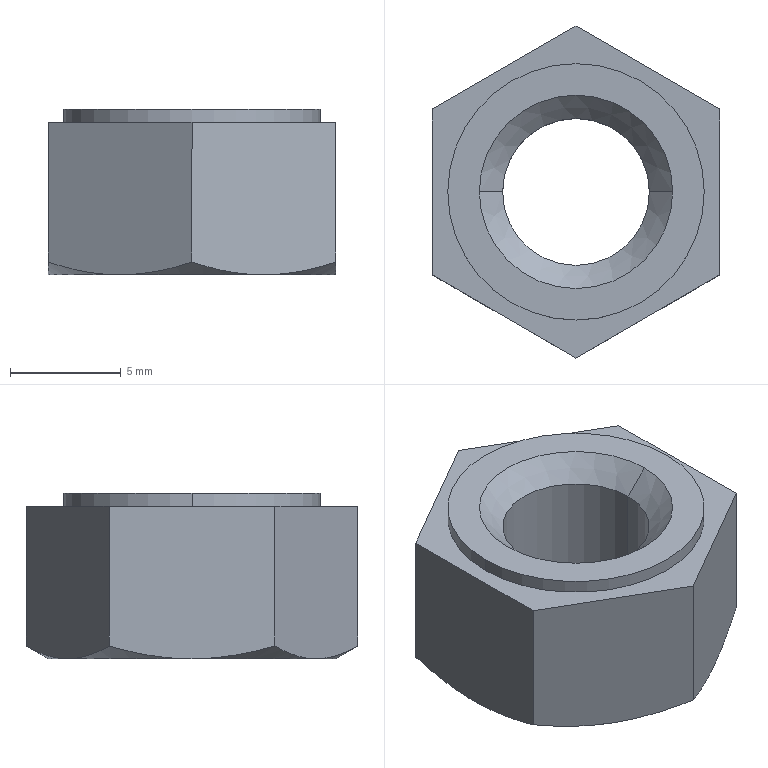Part | SolidWorks | features BaseBody 1 | 1 solid | 23 faces | box 13 x 15.011 x 7.5 mm | volume 785.095 mm3 | cone 10 | plane 9 | cylinder 4 | commonest cylinder face diameters 6.647 x2 11.6 x2
STEP:
#1=CARTESIAN_POINT('',(3.323,0.,1.052));
#2=VERTEX_POINT('',#1);
#3=CARTESIAN_POINT('',(-3.323,0.,1.052));
#4=VERTEX_POINT('',#3);
#5=CARTESIAN_POINT('',(0.,0.,1.052));
#6=DIRECTION('',(0.,0.,-1.));
#7=DIRECTION('',(-1.,0.,0.));
#8=AXIS2_PLACEMENT_3D('',#5,#6,#7);
#9=CIRCLE('',#8,3.323);
#10=EDGE_CURVE('',#2,#4,#9,.T.);
#11=ORIENTED_EDGE('',*,*,#10,.F.);
#12=CARTESIAN_POINT('',(4.375,0.,0.));
#13=VERTEX_POINT('',#12);
#14=CARTESIAN_POINT('',(4.375,0.,0.));
#15=DIRECTION('',(0.7071,0.,-0.7071));
#16=VECTOR('',#15,1000.);
#17=LINE('',#14,#16);
#18=EDGE_CURVE('',#2,#13,#17,.T.);
#19=ORIENTED_EDGE('',*,*,#18,.T.);
#20=CARTESIAN_POINT('',(-4.375,0.,0.));
#21=VERTEX_POINT('',#20);
#22=CARTESIAN_POINT('',(0.,0.,0.));
#23=DIRECTION('',(0.,0.,1.));
#24=DIRECTION('',(-1.,0.,0.));
#25=AXIS2_PLACEMENT_3D('',#22,#23,#24);
#26=CIRCLE('',#25,4.375);
#27=EDGE_CURVE('',#21,#13,#26,.T.);
#28=ORIENTED_EDGE('',*,*,#27,.F.);
#29=CARTESIAN_POINT('',(-4.375,0.,0.));
#30=DIRECTION('',(-0.7071,0.,-0.7071));
#31=VECTOR('',#30,1000.);
#32=LINE('',#29,#31);
#33=EDGE_CURVE('',#4,#21,#32,.T.);
#34=ORIENTED_EDGE('',*,*,#33,.F.);
#35=EDGE_LOOP('',(#11,#19,#28,#34));
#36=FACE_OUTER_BOUND('',#35,.T.);
#37=CARTESIAN_POINT('',(0.,0.,0.));
#38=DIRECTION('',(0.,0.,-1.));
#39=DIRECTION('',(-1.,0.,0.));
#40=AXIS2_PLACEMENT_3D('',#37,#38,#39);
#41=CONICAL_SURFACE('',#40,4.375,0.7854);
#42=ADVANCED_FACE('',(#36),#41,.F.);
#43=CARTESIAN_POINT('',(3.323,0.,6.448));
#44=VERTEX_POINT('',#43);
#45=CARTESIAN_POINT('',(-3.323,0.,6.448));
#46=VERTEX_POINT('',#45);
#47=CARTESIAN_POINT('',(0.,0.,6.448));
#48=DIRECTION('',(0.,0.,-1.));
#49=DIRECTION('',(-1.,0.,0.));
#50=AXIS2_PLACEMENT_3D('',#47,#48,#49);
#51=CIRCLE('',#50,3.323);
#52=EDGE_CURVE('',#44,#46,#51,.T.);
#53=ORIENTED_EDGE('',*,*,#52,.F.);
#54=CARTESIAN_POINT('',(3.323,0.,7.5));
#55=DIRECTION('',(0.,0.,-1.));
#56=VECTOR('',#55,1000.);
#57=LINE('',#54,#56);
#58=EDGE_CURVE('',#44,#2,#57,.T.);
#59=ORIENTED_EDGE('',*,*,#58,.T.);
#60=ORIENTED_EDGE('',*,*,#10,.T.);
#61=CARTESIAN_POINT('',(-3.323,0.,7.5));
#62=DIRECTION('',(0.,0.,-1.));
#63=VECTOR('',#62,1000.);
#64=LINE('',#61,#63);
#65=EDGE_CURVE('',#46,#4,#64,.T.);
#66=ORIENTED_EDGE('',*,*,#65,.F.);
#67=EDGE_LOOP('',(#53,#59,#60,#66));
#68=FACE_OUTER_BOUND('',#67,.T.);
#69=CARTESIAN_POINT('',(0.,0.,7.5));
#70=DIRECTION('',(0.,0.,-1.));
#71=DIRECTION('',(-1.,0.,0.));
#72=AXIS2_PLACEMENT_3D('',#69,#70,#71);
#73=CYLINDRICAL_SURFACE('',#72,3.323);
#74=ADVANCED_FACE('',(#68),#73,.F.);
#75=ORIENTED_EDGE('',*,*,#52,.T.);
#76=CARTESIAN_POINT('',(-4.375,0.,7.5));
#77=VERTEX_POINT('',#76);
#78=CARTESIAN_POINT('',(-4.375,0.,7.5));
#79=DIRECTION('',(-0.7071,0.,0.7071));
#80=VECTOR('',#79,1000.);
#81=LINE('',#78,#80);
#82=EDGE_CURVE('',#46,#77,#81,.T.);
#83=ORIENTED_EDGE('',*,*,#82,.T.);
#84=CARTESIAN_POINT('',(4.375,0.,7.5));
#85=VERTEX_POINT('',#84);
#86=CARTESIAN_POINT('',(0.,0.,7.5));
#87=DIRECTION('',(0.,0.,-1.));
#88=DIRECTION('',(1.,0.,0.));
#89=AXIS2_PLACEMENT_3D('',#86,#87,#88);
#90=CIRCLE('',#89,4.375);
#91=EDGE_CURVE('',#85,#77,#90,.T.);
#92=ORIENTED_EDGE('',*,*,#91,.F.);
#93=CARTESIAN_POINT('',(4.375,0.,7.5));
#94=DIRECTION('',(0.7071,0.,0.7071));
#95=VECTOR('',#94,1000.);
#96=LINE('',#93,#95);
#97=EDGE_CURVE('',#44,#85,#96,.T.);
#98=ORIENTED_EDGE('',*,*,#97,.F.);
#99=EDGE_LOOP('',(#75,#83,#92,#98));
#100=FACE_OUTER_BOUND('',#99,.T.);
#101=CARTESIAN_POINT('',(0.,0.,7.5));
#102=DIRECTION('',(0.,0.,1.));
#103=DIRECTION('',(1.,0.,0.));
#104=AXIS2_PLACEMENT_3D('',#101,#102,#103);
#105=CONICAL_SURFACE('',#104,4.375,0.7854);
#106=ADVANCED_FACE('',(#100),#105,.F.);
#107=CARTESIAN_POINT('',(-5.8,0.,6.9));
#108=VERTEX_POINT('',#107);
#109=CARTESIAN_POINT('',(5.8,0.,6.9));
#110=VERTEX_POINT('',#109);
#111=CARTESIAN_POINT('',(0.,0.,6.9));
#112=DIRECTION('',(0.,0.,-1.));
#113=DIRECTION('',(1.,0.,0.));
#114=AXIS2_PLACEMENT_3D('',#111,#112,#113);
#115=CIRCLE('',#114,5.8);
#116=EDGE_CURVE('',#108,#110,#115,.T.);
#117=ORIENTED_EDGE('',*,*,#116,.F.);
#118=CARTESIAN_POINT('',(-5.8,0.,7.5));
#119=VERTEX_POINT('',#118);
#120=CARTESIAN_POINT('',(-5.8,0.,6.9));
#121=DIRECTION('',(0.,0.,1.));
#122=VECTOR('',#121,1000.);
#123=LINE('',#120,#122);
#124=EDGE_CURVE('',#108,#119,#123,.T.);
#125=ORIENTED_EDGE('',*,*,#124,.T.);
#126=CARTESIAN_POINT('',(5.8,0.,7.5));
#127=VERTEX_POINT('',#126);
#128=CARTESIAN_POINT('',(0.,0.,7.5));
#129=DIRECTION('',(0.,0.,-1.));
#130=DIRECTION('',(1.,0.,0.));
#131=AXIS2_PLACEMENT_3D('',#128,#129,#130);
#132=CIRCLE('',#131,5.8);
#133=EDGE_CURVE('',#119,#127,#132,.T.);
#134=ORIENTED_EDGE('',*,*,#133,.T.);
#135=CARTESIAN_POINT('',(5.8,0.,6.9));
#136=DIRECTION('',(0.,0.,1.));
#137=VECTOR('',#136,1000.);
#138=LINE('',#135,#137);
#139=EDGE_CURVE('',#110,#127,#138,.T.);
#140=ORIENTED_EDGE('',*,*,#139,.F.);
#141=EDGE_LOOP('',(#117,#125,#134,#140));
#142=FACE_OUTER_BOUND('',#141,.T.);
#143=CARTESIAN_POINT('',(0.,0.,6.9));
#144=DIRECTION('',(0.,0.,1.));
#145=DIRECTION('',(1.,0.,0.));
#146=AXIS2_PLACEMENT_3D('',#143,#144,#145);
#147=CYLINDRICAL_SURFACE('',#146,5.8);
#148=ADVANCED_FACE('',(#142),#147,.T.);
#149=CARTESIAN_POINT('',(6.5,0.,0.));
#150=VERTEX_POINT('',#149);
#151=CARTESIAN_POINT('',(3.25,-5.629,0.));
#152=VERTEX_POINT('',#151);
#153=CARTESIAN_POINT('',(0.,0.,0.));
#154=DIRECTION('',(0.,0.,-1.));
#155=DIRECTION('',(1.,0.,0.));
#156=AXIS2_PLACEMENT_3D('',#153,#154,#155);
#157=CIRCLE('',#156,6.5);
#158=EDGE_CURVE('',#150,#152,#157,.T.);
#159=ORIENTED_EDGE('',*,*,#158,.T.);
#160=CARTESIAN_POINT('',(-3.25,-5.629,0.));
#161=VERTEX_POINT('',#160);
#162=CARTESIAN_POINT('',(0.,0.,0.));
#163=DIRECTION('',(0.,0.,-1.));
#164=DIRECTION('',(1.,0.,0.));
#165=AXIS2_PLACEMENT_3D('',#162,#163,#164);
#166=CIRCLE('',#165,6.5);
#167=EDGE_CURVE('',#152,#161,#166,.T.);
#168=ORIENTED_EDGE('',*,*,#167,.T.);
#169=CARTESIAN_POINT('',(-6.5,0.,0.));
#170=VERTEX_POINT('',#169);
#171=CARTESIAN_POINT('',(0.,0.,0.));
#172=DIRECTION('',(0.,0.,-1.));
#173=DIRECTION('',(1.,0.,0.));
#174=AXIS2_PLACEMENT_3D('',#171,#172,#173);
#175=CIRCLE('',#174,6.5);
#176=EDGE_CURVE('',#161,#170,#175,.T.);
#177=ORIENTED_EDGE('',*,*,#176,.T.);
#178=CARTESIAN_POINT('',(-3.25,5.629,0.));
#179=VERTEX_POINT('',#178);
#180=CARTESIAN_POINT('',(0.,0.,0.));
#181=DIRECTION('',(0.,0.,-1.));
#182=DIRECTION('',(1.,0.,0.));
#183=AXIS2_PLACEMENT_3D('',#180,#181,#182);
#184=CIRCLE('',#183,6.5);
#185=EDGE_CURVE('',#170,#179,#184,.T.);
#186=ORIENTED_EDGE('',*,*,#185,.T.);
#187=CARTESIAN_POINT('',(3.25,5.629,0.));
#188=VERTEX_POINT('',#187);
#189=CARTESIAN_POINT('',(0.,0.,0.));
#190=DIRECTION('',(0.,0.,-1.));
#191=DIRECTION('',(1.,0.,0.));
#192=AXIS2_PLACEMENT_3D('',#189,#190,#191);
#193=CIRCLE('',#192,6.5);
#194=EDGE_CURVE('',#179,#188,#193,.T.);
#195=ORIENTED_EDGE('',*,*,#194,.T.);
#196=CARTESIAN_POINT('',(0.,0.,0.));
#197=DIRECTION('',(0.,0.,-1.));
#198=DIRECTION('',(1.,0.,0.));
#199=AXIS2_PLACEMENT_3D('',#196,#197,#198);
#200=CIRCLE('',#199,6.5);
#201=EDGE_CURVE('',#188,#150,#200,.T.);
#202=ORIENTED_EDGE('',*,*,#201,.T.);
#203=EDGE_LOOP('',(#159,#168,#177,#186,#195,#202));
#204=FACE_OUTER_BOUND('',#203,.T.);
#205=ORIENTED_EDGE('',*,*,#27,.T.);
#206=CARTESIAN_POINT('',(0.,0.,0.));
#207=DIRECTION('',(0.,0.,1.));
#208=DIRECTION('',(-1.,0.,0.));
#209=AXIS2_PLACEMENT_3D('',#206,#207,#208);
#210=CIRCLE('',#209,4.375);
#211=EDGE_CURVE('',#13,#21,#210,.T.);
#212=ORIENTED_EDGE('',*,*,#211,.T.);
#213=EDGE_LOOP('',(#205,#212));
#214=FACE_BOUND('',#213,.T.);
#215=CARTESIAN_POINT('',(6.5,3.753,0.));
#216=DIRECTION('',(0.,0.,-1.));
#217=DIRECTION('',(-1.,0.,0.));
#218=AXIS2_PLACEMENT_3D('',#215,#216,#217);
#219=PLANE('',#218);
#220=ADVANCED_FACE('',(#204,#214),#219,.T.);
#221=ORIENTED_EDGE('',*,*,#167,.F.);
#222=CARTESIAN_POINT('',(-0.000000038,-7.506,0.5806));
#223=VERTEX_POINT('',#222);
#224=CARTESIAN_POINT('',(3.25,-5.629,0.));
#225=CARTESIAN_POINT('',(2.141,-6.27,0.));
#226=CARTESIAN_POINT('',(1.062,-6.892,0.2266));
#227=CARTESIAN_POINT('',(-0.000000038,-7.506,0.5806));
#228=B_SPLINE_CURVE_WITH_KNOTS('',3,(#224,#225,#226,#227),.UNSPECIFIED.,.F.,.F.,(4,4),(0.,0.003797),.UNSPECIFIED.);
#229=EDGE_CURVE('',#152,#223,#228,.T.);
#230=ORIENTED_EDGE('',*,*,#229,.T.);
#231=CARTESIAN_POINT('',(-0.000000038,-7.506,0.5806));
#232=CARTESIAN_POINT('',(-1.062,-6.892,0.2266));
#233=CARTESIAN_POINT('',(-2.141,-6.27,0.));
#234=CARTESIAN_POINT('',(-3.25,-5.629,0.));
#235=B_SPLINE_CURVE_WITH_KNOTS('',3,(#231,#232,#233,#234),.UNSPECIFIED.,.F.,.F.,(4,4),(0.,0.003797),.UNSPECIFIED.);
#236=EDGE_CURVE('',#223,#161,#235,.T.);
#237=ORIENTED_EDGE('',*,*,#236,.T.);
#238=EDGE_LOOP('',(#221,#230,#237));
#239=FACE_OUTER_BOUND('',#238,.T.);
#240=CARTESIAN_POINT('',(0.,0.,0.584));
#241=DIRECTION('',(0.,0.,1.));
#242=DIRECTION('',(1.,0.,0.));
#243=AXIS2_PLACEMENT_3D('',#240,#241,#242);
#244=CONICAL_SURFACE('',#243,7.512,1.047);
#245=ADVANCED_FACE('',(#239),#244,.T.);
#246=ORIENTED_EDGE('',*,*,#158,.F.);
#247=CARTESIAN_POINT('',(6.5,-3.753,0.5806));
#248=VERTEX_POINT('',#247);
#249=CARTESIAN_POINT('',(6.5,0.,0.));
#250=CARTESIAN_POINT('',(6.5,-1.281,0.));
#251=CARTESIAN_POINT('',(6.5,-2.527,0.2266));
#252=CARTESIAN_POINT('',(6.5,-3.753,0.5806));
#253=B_SPLINE_CURVE_WITH_KNOTS('',3,(#249,#250,#251,#252),.UNSPECIFIED.,.F.,.F.,(4,4),(0.,0.003797),.UNSPECIFIED.);
#254=EDGE_CURVE('',#150,#248,#253,.T.);
#255=ORIENTED_EDGE('',*,*,#254,.T.);
#256=CARTESIAN_POINT('',(6.5,-3.753,0.5806));
#257=CARTESIAN_POINT('',(5.438,-4.366,0.2266));
#258=CARTESIAN_POINT('',(4.359,-4.989,0.));
#259=CARTESIAN_POINT('',(3.25,-5.629,0.));
#260=B_SPLINE_CURVE_WITH_KNOTS('',3,(#256,#257,#258,#259),.UNSPECIFIED.,.F.,.F.,(4,4),(0.,0.003797),.UNSPECIFIED.);
#261=EDGE_CURVE('',#248,#152,#260,.T.);
#262=ORIENTED_EDGE('',*,*,#261,.T.);
#263=EDGE_LOOP('',(#246,#255,#262));
#264=FACE_OUTER_BOUND('',#263,.T.);
#265=CARTESIAN_POINT('',(0.,0.,0.584));
#266=DIRECTION('',(0.,0.,1.));
#267=DIRECTION('',(1.,0.,0.));
#268=AXIS2_PLACEMENT_3D('',#265,#266,#267);
#269=CONICAL_SURFACE('',#268,7.512,1.047);
#270=ADVANCED_FACE('',(#264),#269,.T.);
#271=CARTESIAN_POINT('',(6.5,3.753,0.5806));
#272=VERTEX_POINT('',#271);
#273=CARTESIAN_POINT('',(6.5,3.753,0.5806));
#274=CARTESIAN_POINT('',(6.5,2.527,0.2266));
#275=CARTESIAN_POINT('',(6.5,1.281,0.));
#276=CARTESIAN_POINT('',(6.5,0.,0.));
#277=B_SPLINE_CURVE_WITH_KNOTS('',3,(#273,#274,#275,#276),.UNSPECIFIED.,.F.,.F.,(4,4),(0.,0.003797),.UNSPECIFIED.);
#278=EDGE_CURVE('',#272,#150,#277,.T.);
#279=ORIENTED_EDGE('',*,*,#278,.T.);
#280=ORIENTED_EDGE('',*,*,#201,.F.);
#281=CARTESIAN_POINT('',(3.25,5.629,0.));
#282=CARTESIAN_POINT('',(4.359,4.989,0.));
#283=CARTESIAN_POINT('',(5.438,4.366,0.2266));
#284=CARTESIAN_POINT('',(6.5,3.753,0.5806));
#285=B_SPLINE_CURVE_WITH_KNOTS('',3,(#281,#282,#283,#284),.UNSPECIFIED.,.F.,.F.,(4,4),(0.,0.003797),.UNSPECIFIED.);
#286=EDGE_CURVE('',#188,#272,#285,.T.);
#287=ORIENTED_EDGE('',*,*,#286,.T.);
#288=EDGE_LOOP('',(#279,#280,#287));
#289=FACE_OUTER_BOUND('',#288,.T.);
#290=CARTESIAN_POINT('',(0.,0.,0.584));
#291=DIRECTION('',(0.,0.,1.));
#292=DIRECTION('',(1.,0.,0.));
#293=AXIS2_PLACEMENT_3D('',#290,#291,#292);
#294=CONICAL_SURFACE('',#293,7.512,1.047);
#295=ADVANCED_FACE('',(#289),#294,.T.);
#296=CARTESIAN_POINT('',(-0.000000014,7.506,0.5806));
#297=VERTEX_POINT('',#296);
#298=CARTESIAN_POINT('',(-0.000000014,7.506,0.5806));
#299=CARTESIAN_POINT('',(1.062,6.892,0.2266));
#300=CARTESIAN_POINT('',(2.141,6.27,0.));
#301=CARTESIAN_POINT('',(3.25,5.629,0.));
#302=B_SPLINE_CURVE_WITH_KNOTS('',3,(#298,#299,#300,#301),.UNSPECIFIED.,.F.,.F.,(4,4),(0.,0.003797),.UNSPECIFIED.);
#303=EDGE_CURVE('',#297,#188,#302,.T.);
#304=ORIENTED_EDGE('',*,*,#303,.T.);
#305=ORIENTED_EDGE('',*,*,#194,.F.);
#306=CARTESIAN_POINT('',(-3.25,5.629,0.));
#307=CARTESIAN_POINT('',(-2.141,6.27,0.));
#308=CARTESIAN_POINT('',(-1.062,6.892,0.2266));
#309=CARTESIAN_POINT('',(-0.000000014,7.506,0.5806));
#310=B_SPLINE_CURVE_WITH_KNOTS('',3,(#306,#307,#308,#309),.UNSPECIFIED.,.F.,.F.,(4,4),(0.,0.003797),.UNSPECIFIED.);
#311=EDGE_CURVE('',#179,#297,#310,.T.);
#312=ORIENTED_EDGE('',*,*,#311,.T.);
#313=EDGE_LOOP('',(#304,#305,#312));
#314=FACE_OUTER_BOUND('',#313,.T.);
#315=CARTESIAN_POINT('',(0.,0.,0.584));
#316=DIRECTION('',(0.,0.,1.));
#317=DIRECTION('',(1.,0.,0.));
#318=AXIS2_PLACEMENT_3D('',#315,#316,#317);
#319=CONICAL_SURFACE('',#318,7.512,1.047);
#320=ADVANCED_FACE('',(#314),#319,.T.);
#321=CARTESIAN_POINT('',(-6.5,3.753,0.5806));
#322=VERTEX_POINT('',#321);
#323=CARTESIAN_POINT('',(-6.5,3.753,0.5806));
#324=CARTESIAN_POINT('',(-5.438,4.366,0.2266));
#325=CARTESIAN_POINT('',(-4.359,4.989,0.));
#326=CARTESIAN_POINT('',(-3.25,5.629,0.));
#327=B_SPLINE_CURVE_WITH_KNOTS('',3,(#323,#324,#325,#326),.UNSPECIFIED.,.F.,.F.,(4,4),(0.,0.003797),.UNSPECIFIED.);
#328=EDGE_CURVE('',#322,#179,#327,.T.);
#329=ORIENTED_EDGE('',*,*,#328,.T.);
#330=ORIENTED_EDGE('',*,*,#185,.F.);
#331=CARTESIAN_POINT('',(-6.5,0.,0.));
#332=CARTESIAN_POINT('',(-6.5,1.281,0.));
#333=CARTESIAN_POINT('',(-6.5,2.527,0.2266));
#334=CARTESIAN_POINT('',(-6.5,3.753,0.5806));
#335=B_SPLINE_CURVE_WITH_KNOTS('',3,(#331,#332,#333,#334),.UNSPECIFIED.,.F.,.F.,(4,4),(0.,0.003797),.UNSPECIFIED.);
#336=EDGE_CURVE('',#170,#322,#335,.T.);
#337=ORIENTED_EDGE('',*,*,#336,.T.);
#338=EDGE_LOOP('',(#329,#330,#337));
#339=FACE_OUTER_BOUND('',#338,.T.);
#340=CARTESIAN_POINT('',(0.,0.,0.584));
#341=DIRECTION('',(0.,0.,1.));
#342=DIRECTION('',(1.,0.,0.));
#343=AXIS2_PLACEMENT_3D('',#340,#341,#342);
#344=CONICAL_SURFACE('',#343,7.512,1.047);
#345=ADVANCED_FACE('',(#339),#344,.T.);
#346=ORIENTED_EDGE('',*,*,#176,.F.);
#347=CARTESIAN_POINT('',(-6.5,-3.753,0.5806));
#348=VERTEX_POINT('',#347);
#349=CARTESIAN_POINT('',(-3.25,-5.629,0.));
#350=CARTESIAN_POINT('',(-4.359,-4.989,0.));
#351=CARTESIAN_POINT('',(-5.438,-4.366,0.2266));
#352=CARTESIAN_POINT('',(-6.5,-3.753,0.5806));
#353=B_SPLINE_CURVE_WITH_KNOTS('',3,(#349,#350,#351,#352),.UNSPECIFIED.,.F.,.F.,(4,4),(0.,0.003797),.UNSPECIFIED.);
#354=EDGE_CURVE('',#161,#348,#353,.T.);
#355=ORIENTED_EDGE('',*,*,#354,.T.);
#356=CARTESIAN_POINT('',(-6.5,-3.753,0.5806));
#357=CARTESIAN_POINT('',(-6.5,-2.527,0.2266));
#358=CARTESIAN_POINT('',(-6.5,-1.281,0.));
#359=CARTESIAN_POINT('',(-6.5,0.,0.));
#360=B_SPLINE_CURVE_WITH_KNOTS('',3,(#356,#357,#358,#359),.UNSPECIFIED.,.F.,.F.,(4,4),(0.,0.003797),.UNSPECIFIED.);
#361=EDGE_CURVE('',#348,#170,#360,.T.);
#362=ORIENTED_EDGE('',*,*,#361,.T.);
#363=EDGE_LOOP('',(#346,#355,#362));
#364=FACE_OUTER_BOUND('',#363,.T.);
#365=CARTESIAN_POINT('',(0.,0.,0.584));
#366=DIRECTION('',(0.,0.,1.));
#367=DIRECTION('',(1.,0.,0.));
#368=AXIS2_PLACEMENT_3D('',#365,#366,#367);
#369=CONICAL_SURFACE('',#368,7.512,1.047);
#370=ADVANCED_FACE('',(#364),#369,.T.);
#371=ORIENTED_EDGE('',*,*,#18,.F.);
#372=CARTESIAN_POINT('',(0.,0.,1.052));
#373=DIRECTION('',(0.,0.,-1.));
#374=DIRECTION('',(-1.,0.,0.));
#375=AXIS2_PLACEMENT_3D('',#372,#373,#374);
#376=CIRCLE('',#375,3.323);
#377=EDGE_CURVE('',#4,#2,#376,.T.);
#378=ORIENTED_EDGE('',*,*,#377,.F.);
#379=ORIENTED_EDGE('',*,*,#33,.T.);
#380=ORIENTED_EDGE('',*,*,#211,.F.);
#381=EDGE_LOOP('',(#371,#378,#379,#380));
#382=FACE_OUTER_BOUND('',#381,.T.);
#383=CARTESIAN_POINT('',(0.,0.,0.));
#384=DIRECTION('',(0.,0.,-1.));
#385=DIRECTION('',(-1.,0.,0.));
#386=AXIS2_PLACEMENT_3D('',#383,#384,#385);
#387=CONICAL_SURFACE('',#386,4.375,0.7854);
#388=ADVANCED_FACE('',(#382),#387,.F.);
#389=CARTESIAN_POINT('',(0.,-7.506,6.9));
#390=VERTEX_POINT('',#389);
#391=CARTESIAN_POINT('',(0.,-7.506,7.5));
#392=DIRECTION('',(0.,0.,1.));
#393=VECTOR('',#392,1000.);
#394=LINE('',#391,#393);
#395=EDGE_CURVE('',#223,#390,#394,.T.);
#396=ORIENTED_EDGE('',*,*,#395,.F.);
#397=ORIENTED_EDGE('',*,*,#229,.F.);
#398=ORIENTED_EDGE('',*,*,#261,.F.);
#399=CARTESIAN_POINT('',(6.5,-3.753,6.9));
#400=VERTEX_POINT('',#399);
#401=CARTESIAN_POINT('',(6.5,-3.753,7.5));
#402=DIRECTION('',(0.,0.,-1.));
#403=VECTOR('',#402,1000.);
#404=LINE('',#401,#403);
#405=EDGE_CURVE('',#400,#248,#404,.T.);
#406=ORIENTED_EDGE('',*,*,#405,.F.);
#407=CARTESIAN_POINT('',(0.,-7.506,6.9));
#408=DIRECTION('',(0.866,0.5,0.));
#409=VECTOR('',#408,1000.);
#410=LINE('',#407,#409);
#411=EDGE_CURVE('',#390,#400,#410,.T.);
#412=ORIENTED_EDGE('',*,*,#411,.F.);
#413=EDGE_LOOP('',(#396,#397,#398,#406,#412));
#414=FACE_OUTER_BOUND('',#413,.T.);
#415=CARTESIAN_POINT('',(0.,-7.506,7.5));
#416=DIRECTION('',(-0.5,0.866,0.));
#417=DIRECTION('',(-0.866,-0.5,0.));
#418=AXIS2_PLACEMENT_3D('',#415,#416,#417);
#419=PLANE('',#418);
#420=ADVANCED_FACE('',(#414),#419,.F.);
#421=CARTESIAN_POINT('',(-6.5,-3.753,6.9));
#422=VERTEX_POINT('',#421);
#423=CARTESIAN_POINT('',(-6.5,-3.753,7.5));
#424=DIRECTION('',(0.,0.,1.));
#425=VECTOR('',#424,1000.);
#426=LINE('',#423,#425);
#427=EDGE_CURVE('',#348,#422,#426,.T.);
#428=ORIENTED_EDGE('',*,*,#427,.F.);
#429=ORIENTED_EDGE('',*,*,#354,.F.);
#430=ORIENTED_EDGE('',*,*,#236,.F.);
#431=ORIENTED_EDGE('',*,*,#395,.T.);
#432=CARTESIAN_POINT('',(-6.5,-3.753,6.9));
#433=DIRECTION('',(0.866,-0.5,0.));
#434=VECTOR('',#433,1000.);
#435=LINE('',#432,#434);
#436=EDGE_CURVE('',#422,#390,#435,.T.);
#437=ORIENTED_EDGE('',*,*,#436,.F.);
#438=EDGE_LOOP('',(#428,#429,#430,#431,#437));
#439=FACE_OUTER_BOUND('',#438,.T.);
#440=CARTESIAN_POINT('',(-6.5,-3.753,7.5));
#441=DIRECTION('',(0.5,0.866,0.));
#442=DIRECTION('',(-0.866,0.5,0.));
#443=AXIS2_PLACEMENT_3D('',#440,#441,#442);
#444=PLANE('',#443);
#445=ADVANCED_FACE('',(#439),#444,.F.);
#446=ORIENTED_EDGE('',*,*,#405,.T.);
#447=ORIENTED_EDGE('',*,*,#254,.F.);
#448=ORIENTED_EDGE('',*,*,#278,.F.);
#449=CARTESIAN_POINT('',(6.5,3.753,6.9));
#450=VERTEX_POINT('',#449);
#451=CARTESIAN_POINT('',(6.5,3.753,7.5));
#452=DIRECTION('',(0.,0.,-1.));
#453=VECTOR('',#452,1000.);
#454=LINE('',#451,#453);
#455=EDGE_CURVE('',#450,#272,#454,.T.);
#456=ORIENTED_EDGE('',*,*,#455,.F.);
#457=CARTESIAN_POINT('',(6.5,-3.753,6.9));
#458=DIRECTION('',(0.,1.,0.));
#459=VECTOR('',#458,1000.);
#460=LINE('',#457,#459);
#461=EDGE_CURVE('',#400,#450,#460,.T.);
#462=ORIENTED_EDGE('',*,*,#461,.F.);
#463=EDGE_LOOP('',(#446,#447,#448,#456,#462));
#464=FACE_OUTER_BOUND('',#463,.T.);
#465=CARTESIAN_POINT('',(6.5,-3.753,7.5));
#466=DIRECTION('',(-1.,0.,0.));
#467=DIRECTION('',(0.,-1.,0.));
#468=AXIS2_PLACEMENT_3D('',#465,#466,#467);
#469=PLANE('',#468);
#470=ADVANCED_FACE('',(#464),#469,.F.);
#471=ORIENTED_EDGE('',*,*,#455,.T.);
#472=ORIENTED_EDGE('',*,*,#286,.F.);
#473=ORIENTED_EDGE('',*,*,#303,.F.);
#474=CARTESIAN_POINT('',(0.,7.506,6.9));
#475=VERTEX_POINT('',#474);
#476=CARTESIAN_POINT('',(0.,7.506,7.5));
#477=DIRECTION('',(0.,0.,-1.));
#478=VECTOR('',#477,1000.);
#479=LINE('',#476,#478);
#480=EDGE_CURVE('',#475,#297,#479,.T.);
#481=ORIENTED_EDGE('',*,*,#480,.F.);
#482=CARTESIAN_POINT('',(6.5,3.753,6.9));
#483=DIRECTION('',(-0.866,0.5,0.));
#484=VECTOR('',#483,1000.);
#485=LINE('',#482,#484);
#486=EDGE_CURVE('',#450,#475,#485,.T.);
#487=ORIENTED_EDGE('',*,*,#486,.F.);
#488=EDGE_LOOP('',(#471,#472,#473,#481,#487));
#489=FACE_OUTER_BOUND('',#488,.T.);
#490=CARTESIAN_POINT('',(6.5,3.753,7.5));
#491=DIRECTION('',(-0.5,-0.866,0.));
#492=DIRECTION('',(0.866,-0.5,0.));
#493=AXIS2_PLACEMENT_3D('',#490,#491,#492);
#494=PLANE('',#493);
#495=ADVANCED_FACE('',(#489),#494,.F.);
#496=ORIENTED_EDGE('',*,*,#480,.T.);
#497=ORIENTED_EDGE('',*,*,#311,.F.);
#498=ORIENTED_EDGE('',*,*,#328,.F.);
#499=CARTESIAN_POINT('',(-6.5,3.753,6.9));
#500=VERTEX_POINT('',#499);
#501=CARTESIAN_POINT('',(-6.5,3.753,7.5));
#502=DIRECTION('',(0.,0.,-1.));
#503=VECTOR('',#502,1000.);
#504=LINE('',#501,#503);
#505=EDGE_CURVE('',#500,#322,#504,.T.);
#506=ORIENTED_EDGE('',*,*,#505,.F.);
#507=CARTESIAN_POINT('',(0.,7.506,6.9));
#508=DIRECTION('',(-0.866,-0.5,0.));
#509=VECTOR('',#508,1000.);
#510=LINE('',#507,#509);
#511=EDGE_CURVE('',#475,#500,#510,.T.);
#512=ORIENTED_EDGE('',*,*,#511,.F.);
#513=EDGE_LOOP('',(#496,#497,#498,#506,#512));
#514=FACE_OUTER_BOUND('',#513,.T.);
#515=CARTESIAN_POINT('',(0.,7.506,7.5));
#516=DIRECTION('',(0.5,-0.866,0.));
#517=DIRECTION('',(0.866,0.5,0.));
#518=AXIS2_PLACEMENT_3D('',#515,#516,#517);
#519=PLANE('',#518);
#520=ADVANCED_FACE('',(#514),#519,.F.);
#521=ORIENTED_EDGE('',*,*,#505,.T.);
#522=ORIENTED_EDGE('',*,*,#336,.F.);
#523=ORIENTED_EDGE('',*,*,#361,.F.);
#524=ORIENTED_EDGE('',*,*,#427,.T.);
#525=CARTESIAN_POINT('',(-6.5,3.753,6.9));
#526=DIRECTION('',(0.,-1.,0.));
#527=VECTOR('',#526,1000.);
#528=LINE('',#525,#527);
#529=EDGE_CURVE('',#500,#422,#528,.T.);
#530=ORIENTED_EDGE('',*,*,#529,.F.);
#531=EDGE_LOOP('',(#521,#522,#523,#524,#530));
#532=FACE_OUTER_BOUND('',#531,.T.);
#533=CARTESIAN_POINT('',(-6.5,3.753,7.5));
#534=DIRECTION('',(1.,0.,0.));
#535=DIRECTION('',(0.,1.,0.));
#536=AXIS2_PLACEMENT_3D('',#533,#534,#535);
#537=PLANE('',#536);
#538=ADVANCED_FACE('',(#532),#537,.F.);
#539=ORIENTED_EDGE('',*,*,#58,.F.);
#540=CARTESIAN_POINT('',(0.,0.,6.448));
#541=DIRECTION('',(0.,0.,-1.));
#542=DIRECTION('',(-1.,0.,0.));
#543=AXIS2_PLACEMENT_3D('',#540,#541,#542);
#544=CIRCLE('',#543,3.323);
#545=EDGE_CURVE('',#46,#44,#544,.T.);
#546=ORIENTED_EDGE('',*,*,#545,.F.);
#547=ORIENTED_EDGE('',*,*,#65,.T.);
#548=ORIENTED_EDGE('',*,*,#377,.T.);
#549=EDGE_LOOP('',(#539,#546,#547,#548));
#550=FACE_OUTER_BOUND('',#549,.T.);
#551=CARTESIAN_POINT('',(0.,0.,7.5));
#552=DIRECTION('',(0.,0.,-1.));
#553=DIRECTION('',(-1.,0.,0.));
#554=AXIS2_PLACEMENT_3D('',#551,#552,#553);
#555=CYLINDRICAL_SURFACE('',#554,3.323);
#556=ADVANCED_FACE('',(#550),#555,.F.);
#557=ORIENTED_EDGE('',*,*,#411,.T.);
#558=ORIENTED_EDGE('',*,*,#461,.T.);
#559=ORIENTED_EDGE('',*,*,#486,.T.);
#560=ORIENTED_EDGE('',*,*,#511,.T.);
#561=ORIENTED_EDGE('',*,*,#529,.T.);
#562=ORIENTED_EDGE('',*,*,#436,.T.);
#563=EDGE_LOOP('',(#557,#558,#559,#560,#561,#562));
#564=FACE_OUTER_BOUND('',#563,.T.);
#565=CARTESIAN_POINT('',(0.,0.,6.9));
#566=DIRECTION('',(0.,0.,-1.));
#567=DIRECTION('',(1.,0.,0.));
#568=AXIS2_PLACEMENT_3D('',#565,#566,#567);
#569=CIRCLE('',#568,5.8);
#570=EDGE_CURVE('',#110,#108,#569,.T.);
#571=ORIENTED_EDGE('',*,*,#570,.T.);
#572=ORIENTED_EDGE('',*,*,#116,.T.);
#573=EDGE_LOOP('',(#571,#572));
#574=FACE_BOUND('',#573,.T.);
#575=CARTESIAN_POINT('',(0.,0.,6.9));
#576=DIRECTION('',(0.,0.,1.));
#577=DIRECTION('',(1.,0.,0.));
#578=AXIS2_PLACEMENT_3D('',#575,#576,#577);
#579=PLANE('',#578);
#580=ADVANCED_FACE('',(#564,#574),#579,.T.);
#581=ORIENTED_EDGE('',*,*,#82,.F.);
#582=ORIENTED_EDGE('',*,*,#545,.T.);
#583=ORIENTED_EDGE('',*,*,#97,.T.);
#584=CARTESIAN_POINT('',(0.,0.,7.5));
#585=DIRECTION('',(0.,0.,-1.));
#586=DIRECTION('',(1.,0.,0.));
#587=AXIS2_PLACEMENT_3D('',#584,#585,#586);
#588=CIRCLE('',#587,4.375);
#589=EDGE_CURVE('',#77,#85,#588,.T.);
#590=ORIENTED_EDGE('',*,*,#589,.F.);
#591=EDGE_LOOP('',(#581,#582,#583,#590));
#592=FACE_OUTER_BOUND('',#591,.T.);
#593=CARTESIAN_POINT('',(0.,0.,7.5));
#594=DIRECTION('',(0.,0.,1.));
#595=DIRECTION('',(1.,0.,0.));
#596=AXIS2_PLACEMENT_3D('',#593,#594,#595);
#597=CONICAL_SURFACE('',#596,4.375,0.7854);
#598=ADVANCED_FACE('',(#592),#597,.F.);
#599=ORIENTED_EDGE('',*,*,#124,.F.);
#600=ORIENTED_EDGE('',*,*,#570,.F.);
#601=ORIENTED_EDGE('',*,*,#139,.T.);
#602=CARTESIAN_POINT('',(0.,0.,7.5));
#603=DIRECTION('',(0.,0.,-1.));
#604=DIRECTION('',(1.,0.,0.));
#605=AXIS2_PLACEMENT_3D('',#602,#603,#604);
#606=CIRCLE('',#605,5.8);
#607=EDGE_CURVE('',#127,#119,#606,.T.);
#608=ORIENTED_EDGE('',*,*,#607,.T.);
#609=EDGE_LOOP('',(#599,#600,#601,#608));
#610=FACE_OUTER_BOUND('',#609,.T.);
#611=CARTESIAN_POINT('',(0.,0.,6.9));
#612=DIRECTION('',(0.,0.,1.));
#613=DIRECTION('',(1.,0.,0.));
#614=AXIS2_PLACEMENT_3D('',#611,#612,#613);
#615=CYLINDRICAL_SURFACE('',#614,5.8);
#616=ADVANCED_FACE('',(#610),#615,.T.);
#617=ORIENTED_EDGE('',*,*,#607,.F.);
#618=ORIENTED_EDGE('',*,*,#133,.F.);
#619=EDGE_LOOP('',(#617,#618));
#620=FACE_OUTER_BOUND('',#619,.T.);
#621=ORIENTED_EDGE('',*,*,#91,.T.);
#622=ORIENTED_EDGE('',*,*,#589,.T.);
#623=EDGE_LOOP('',(#621,#622));
#624=FACE_BOUND('',#623,.T.);
#625=CARTESIAN_POINT('',(6.5,3.753,7.5));
#626=DIRECTION('',(0.,0.,-1.));
#627=DIRECTION('',(-1.,0.,0.));
#628=AXIS2_PLACEMENT_3D('',#625,#626,#627);
#629=PLANE('',#628);
#630=ADVANCED_FACE('',(#620,#624),#629,.F.);
#631=CLOSED_SHELL('',(#42,#74,#106,#148,#220,#245,#270,#295,#320,#345,#370,#388,#420,#445,#470,#495,#520,#538,#556,#580,#598,#616,#630));
#632=MANIFOLD_SOLID_BREP('',#631);
#633=CARTESIAN_POINT('',(0.,0.,0.));
#634=DIRECTION('',(0.,0.,1.));
#635=DIRECTION('',(1.,0.,0.));
#636=AXIS2_PLACEMENT_3D('',#633,#634,#635);
#637=(LENGTH_UNIT()NAMED_UNIT(*)SI_UNIT(.MILLI.,.METRE.));
#638=UNCERTAINTY_MEASURE_WITH_UNIT(LENGTH_MEASURE(0.00001),#637,'','');
#639=(NAMED_UNIT(*)PLANE_ANGLE_UNIT()SI_UNIT($,.RADIAN.));
#640=(NAMED_UNIT(*)SI_UNIT($,.STERADIAN.)SOLID_ANGLE_UNIT());
#641=(GEOMETRIC_REPRESENTATION_CONTEXT(3)GLOBAL_UNCERTAINTY_ASSIGNED_CONTEXT((#638))GLOBAL_UNIT_ASSIGNED_CONTEXT((#637,#639,#640))REPRESENTATION_CONTEXT('',''));
#642=ADVANCED_BREP_SHAPE_REPRESENTATION('',(#632,#636),#641);